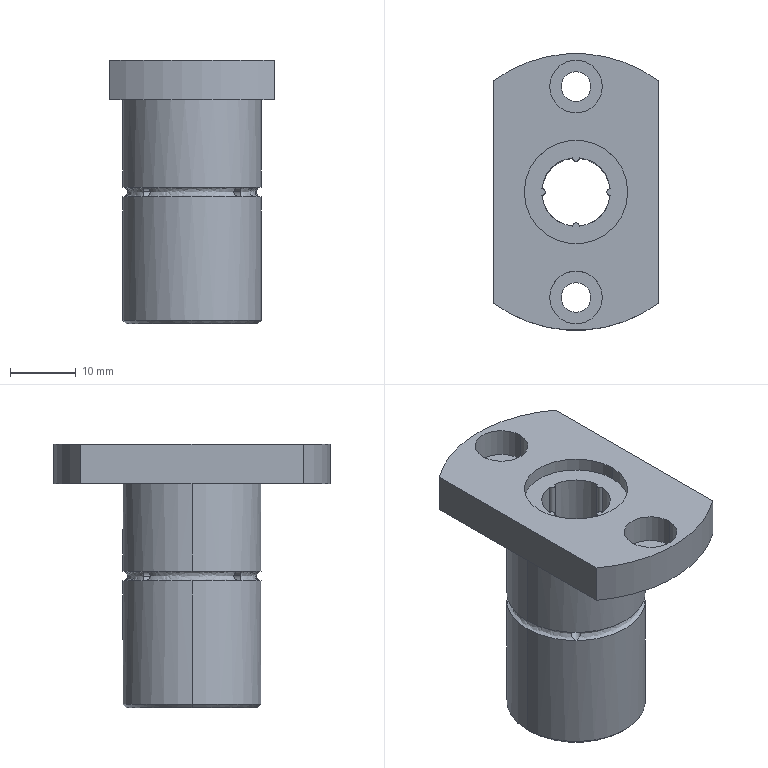Part | SolidWorks | features BaseBody 1 | 1 solid | 51 faces | box 25 x 42 x 40 mm | volume 13318 mm3 | cylinder 35 | plane 9 | spline 5 | cone 2 | commonest cylinder face diameters 1.5 x8 1.04 x5 4.5 x4 8 x4 10.4 x4 15.7 x4